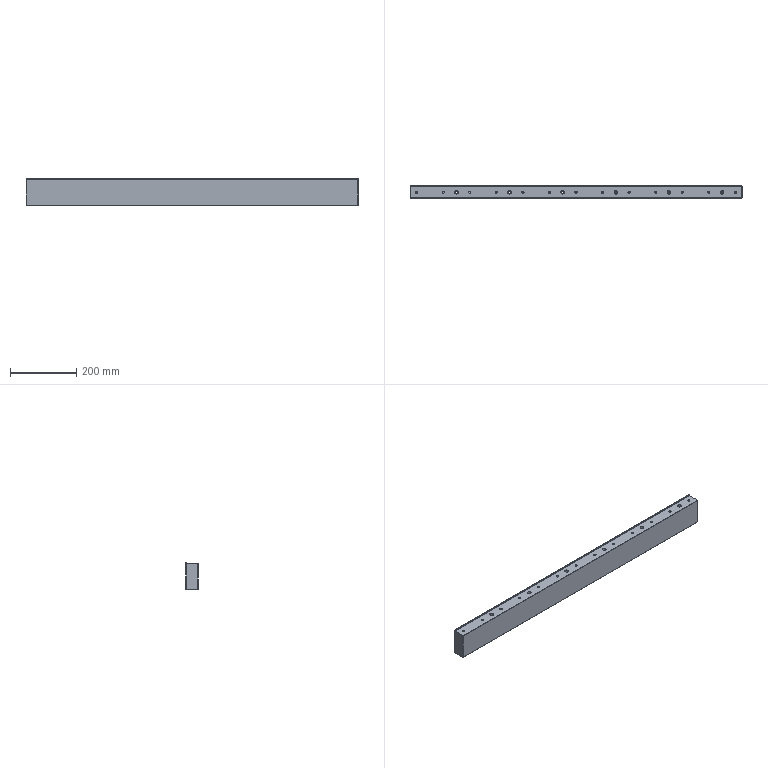Part | STEP file | TJ-DHQM-004-002 | 1 solid | 114 faces | box 1000 x 37.5 x 82.5 mm | volume 2965048 mm3 | cylinder 50 | plane 38 | cone 26 | commonest cylinder face diameters 6.8 x26 6.6 x12 11 x12